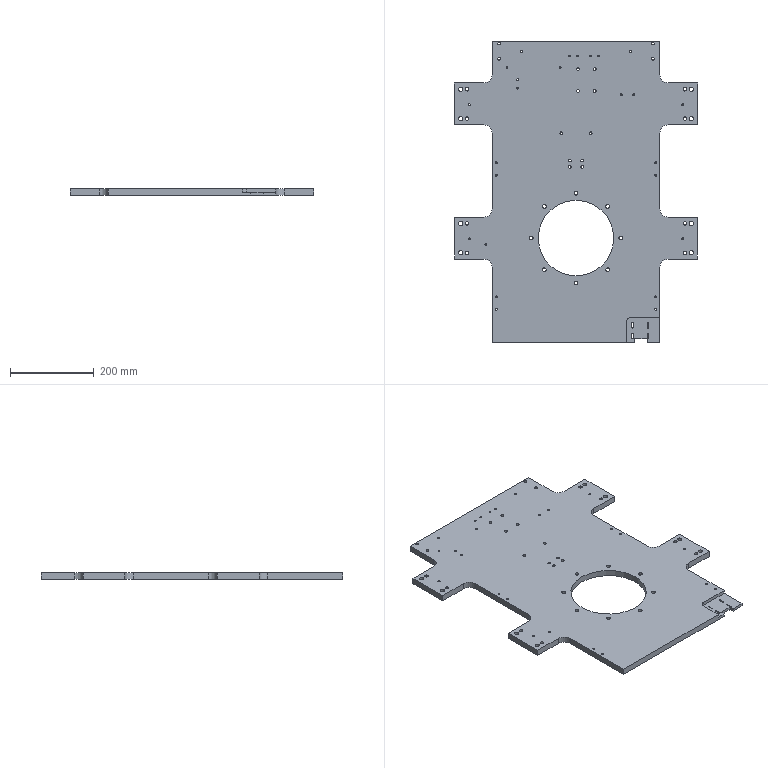Part | NX | features 5003_201_Base plate 2 | 1 solid | 135 faces | box 580 x 720 x 15 mm | volume 4306044 mm3 | cylinder 88 | plane 43 | cone 4 | commonest cylinder face diameters 4.2 x12 5 x10 6.6 x10 3.2 x8 8.376 x8 9 x8